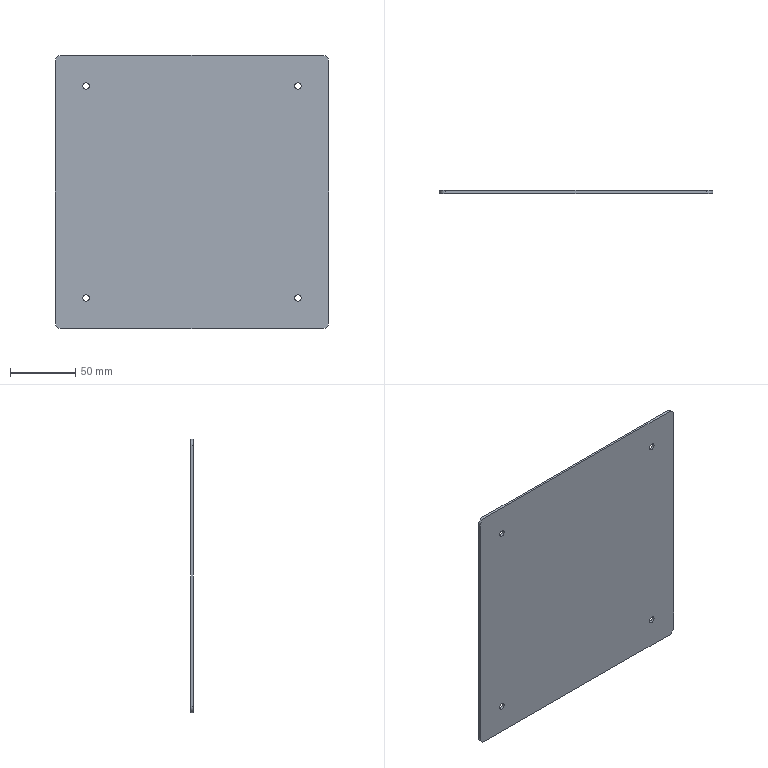Part | SolidWorks | features Extrusion 1, Fillet 1, HoleWzd 1 | 1 solid | 18 faces | box 210 x 2 x 210 mm | volume 88000 mm3 | cylinder 12 | plane 6 | commonest cylinder face diameters 5 x8 10 x4
STEP:
#1=CARTESIAN_POINT('',(-81.317,0.,78.817));
#2=VERTEX_POINT('',#1);
#3=CARTESIAN_POINT('',(-81.317,0.,83.817));
#4=VERTEX_POINT('',#3);
#5=CARTESIAN_POINT('',(-81.317,0.,81.317));
#6=DIRECTION('',(0.,1.,0.));
#7=DIRECTION('',(0.,0.,1.));
#8=AXIS2_PLACEMENT_3D('',#5,#6,#7);
#9=CIRCLE('',#8,2.5);
#10=EDGE_CURVE('',#2,#4,#9,.T.);
#11=ORIENTED_EDGE('',*,*,#10,.F.);
#12=CARTESIAN_POINT('',(-81.317,2.,78.817));
#13=VERTEX_POINT('',#12);
#14=CARTESIAN_POINT('',(-81.317,2.,78.817));
#15=DIRECTION('',(0.,1.,0.));
#16=VECTOR('',#15,1000.);
#17=LINE('',#14,#16);
#18=EDGE_CURVE('',#2,#13,#17,.T.);
#19=ORIENTED_EDGE('',*,*,#18,.T.);
#20=CARTESIAN_POINT('',(-81.317,2.,83.817));
#21=VERTEX_POINT('',#20);
#22=CARTESIAN_POINT('',(-81.317,2.,81.317));
#23=DIRECTION('',(0.,1.,0.));
#24=DIRECTION('',(0.,0.,1.));
#25=AXIS2_PLACEMENT_3D('',#22,#23,#24);
#26=CIRCLE('',#25,2.5);
#27=EDGE_CURVE('',#13,#21,#26,.T.);
#28=ORIENTED_EDGE('',*,*,#27,.T.);
#29=CARTESIAN_POINT('',(-81.317,2.,83.817));
#30=DIRECTION('',(0.,1.,0.));
#31=VECTOR('',#30,1000.);
#32=LINE('',#29,#31);
#33=EDGE_CURVE('',#4,#21,#32,.T.);
#34=ORIENTED_EDGE('',*,*,#33,.F.);
#35=EDGE_LOOP('',(#11,#19,#28,#34));
#36=FACE_OUTER_BOUND('',#35,.T.);
#37=CARTESIAN_POINT('',(-81.317,2.,81.317));
#38=DIRECTION('',(0.,1.,0.));
#39=DIRECTION('',(0.,0.,1.));
#40=AXIS2_PLACEMENT_3D('',#37,#38,#39);
#41=CYLINDRICAL_SURFACE('',#40,2.5);
#42=ADVANCED_FACE('',(#36),#41,.F.);
#43=CARTESIAN_POINT('',(-81.317,0.,-83.817));
#44=VERTEX_POINT('',#43);
#45=CARTESIAN_POINT('',(-81.317,0.,-78.817));
#46=VERTEX_POINT('',#45);
#47=CARTESIAN_POINT('',(-81.317,0.,-81.317));
#48=DIRECTION('',(0.,1.,0.));
#49=DIRECTION('',(0.,0.,1.));
#50=AXIS2_PLACEMENT_3D('',#47,#48,#49);
#51=CIRCLE('',#50,2.5);
#52=EDGE_CURVE('',#44,#46,#51,.T.);
#53=ORIENTED_EDGE('',*,*,#52,.F.);
#54=CARTESIAN_POINT('',(-81.317,2.,-83.817));
#55=VERTEX_POINT('',#54);
#56=CARTESIAN_POINT('',(-81.317,2.,-83.817));
#57=DIRECTION('',(0.,1.,0.));
#58=VECTOR('',#57,1000.);
#59=LINE('',#56,#58);
#60=EDGE_CURVE('',#44,#55,#59,.T.);
#61=ORIENTED_EDGE('',*,*,#60,.T.);
#62=CARTESIAN_POINT('',(-81.317,2.,-78.817));
#63=VERTEX_POINT('',#62);
#64=CARTESIAN_POINT('',(-81.317,2.,-81.317));
#65=DIRECTION('',(0.,1.,0.));
#66=DIRECTION('',(0.,0.,1.));
#67=AXIS2_PLACEMENT_3D('',#64,#65,#66);
#68=CIRCLE('',#67,2.5);
#69=EDGE_CURVE('',#55,#63,#68,.T.);
#70=ORIENTED_EDGE('',*,*,#69,.T.);
#71=CARTESIAN_POINT('',(-81.317,2.,-78.817));
#72=DIRECTION('',(0.,1.,0.));
#73=VECTOR('',#72,1000.);
#74=LINE('',#71,#73);
#75=EDGE_CURVE('',#46,#63,#74,.T.);
#76=ORIENTED_EDGE('',*,*,#75,.F.);
#77=EDGE_LOOP('',(#53,#61,#70,#76));
#78=FACE_OUTER_BOUND('',#77,.T.);
#79=CARTESIAN_POINT('',(-81.317,2.,-81.317));
#80=DIRECTION('',(0.,1.,0.));
#81=DIRECTION('',(0.,0.,1.));
#82=AXIS2_PLACEMENT_3D('',#79,#80,#81);
#83=CYLINDRICAL_SURFACE('',#82,2.5);
#84=ADVANCED_FACE('',(#78),#83,.F.);
#85=CARTESIAN_POINT('',(81.317,0.,-83.817));
#86=VERTEX_POINT('',#85);
#87=CARTESIAN_POINT('',(81.317,0.,-78.817));
#88=VERTEX_POINT('',#87);
#89=CARTESIAN_POINT('',(81.317,0.,-81.317));
#90=DIRECTION('',(0.,1.,0.));
#91=DIRECTION('',(0.,0.,1.));
#92=AXIS2_PLACEMENT_3D('',#89,#90,#91);
#93=CIRCLE('',#92,2.5);
#94=EDGE_CURVE('',#86,#88,#93,.T.);
#95=ORIENTED_EDGE('',*,*,#94,.F.);
#96=CARTESIAN_POINT('',(81.317,2.,-83.817));
#97=VERTEX_POINT('',#96);
#98=CARTESIAN_POINT('',(81.317,2.,-83.817));
#99=DIRECTION('',(0.,1.,0.));
#100=VECTOR('',#99,1000.);
#101=LINE('',#98,#100);
#102=EDGE_CURVE('',#86,#97,#101,.T.);
#103=ORIENTED_EDGE('',*,*,#102,.T.);
#104=CARTESIAN_POINT('',(81.317,2.,-78.817));
#105=VERTEX_POINT('',#104);
#106=CARTESIAN_POINT('',(81.317,2.,-81.317));
#107=DIRECTION('',(0.,1.,0.));
#108=DIRECTION('',(0.,0.,1.));
#109=AXIS2_PLACEMENT_3D('',#106,#107,#108);
#110=CIRCLE('',#109,2.5);
#111=EDGE_CURVE('',#97,#105,#110,.T.);
#112=ORIENTED_EDGE('',*,*,#111,.T.);
#113=CARTESIAN_POINT('',(81.317,2.,-78.817));
#114=DIRECTION('',(0.,1.,0.));
#115=VECTOR('',#114,1000.);
#116=LINE('',#113,#115);
#117=EDGE_CURVE('',#88,#105,#116,.T.);
#118=ORIENTED_EDGE('',*,*,#117,.F.);
#119=EDGE_LOOP('',(#95,#103,#112,#118));
#120=FACE_OUTER_BOUND('',#119,.T.);
#121=CARTESIAN_POINT('',(81.317,2.,-81.317));
#122=DIRECTION('',(0.,1.,0.));
#123=DIRECTION('',(0.,0.,1.));
#124=AXIS2_PLACEMENT_3D('',#121,#122,#123);
#125=CYLINDRICAL_SURFACE('',#124,2.5);
#126=ADVANCED_FACE('',(#120),#125,.F.);
#127=CARTESIAN_POINT('',(81.317,0.,78.817));
#128=VERTEX_POINT('',#127);
#129=CARTESIAN_POINT('',(81.317,0.,83.817));
#130=VERTEX_POINT('',#129);
#131=CARTESIAN_POINT('',(81.317,0.,81.317));
#132=DIRECTION('',(0.,1.,0.));
#133=DIRECTION('',(0.,0.,1.));
#134=AXIS2_PLACEMENT_3D('',#131,#132,#133);
#135=CIRCLE('',#134,2.5);
#136=EDGE_CURVE('',#128,#130,#135,.T.);
#137=ORIENTED_EDGE('',*,*,#136,.F.);
#138=CARTESIAN_POINT('',(81.317,2.,78.817));
#139=VERTEX_POINT('',#138);
#140=CARTESIAN_POINT('',(81.317,2.,78.817));
#141=DIRECTION('',(0.,1.,0.));
#142=VECTOR('',#141,1000.);
#143=LINE('',#140,#142);
#144=EDGE_CURVE('',#128,#139,#143,.T.);
#145=ORIENTED_EDGE('',*,*,#144,.T.);
#146=CARTESIAN_POINT('',(81.317,2.,83.817));
#147=VERTEX_POINT('',#146);
#148=CARTESIAN_POINT('',(81.317,2.,81.317));
#149=DIRECTION('',(0.,1.,0.));
#150=DIRECTION('',(0.,0.,1.));
#151=AXIS2_PLACEMENT_3D('',#148,#149,#150);
#152=CIRCLE('',#151,2.5);
#153=EDGE_CURVE('',#139,#147,#152,.T.);
#154=ORIENTED_EDGE('',*,*,#153,.T.);
#155=CARTESIAN_POINT('',(81.317,2.,83.817));
#156=DIRECTION('',(0.,1.,0.));
#157=VECTOR('',#156,1000.);
#158=LINE('',#155,#157);
#159=EDGE_CURVE('',#130,#147,#158,.T.);
#160=ORIENTED_EDGE('',*,*,#159,.F.);
#161=EDGE_LOOP('',(#137,#145,#154,#160));
#162=FACE_OUTER_BOUND('',#161,.T.);
#163=CARTESIAN_POINT('',(81.317,2.,81.317));
#164=DIRECTION('',(0.,1.,0.));
#165=DIRECTION('',(0.,0.,1.));
#166=AXIS2_PLACEMENT_3D('',#163,#164,#165);
#167=CYLINDRICAL_SURFACE('',#166,2.5);
#168=ADVANCED_FACE('',(#162),#167,.F.);
#169=CARTESIAN_POINT('',(105.,2.,100.));
#170=VERTEX_POINT('',#169);
#171=CARTESIAN_POINT('',(105.,2.,-100.));
#172=VERTEX_POINT('',#171);
#173=CARTESIAN_POINT('',(105.,2.,-105.));
#174=DIRECTION('',(0.,0.,-1.));
#175=VECTOR('',#174,1000.);
#176=LINE('',#173,#175);
#177=EDGE_CURVE('',#170,#172,#176,.T.);
#178=ORIENTED_EDGE('',*,*,#177,.F.);
#179=CARTESIAN_POINT('',(105.,0.,100.));
#180=VERTEX_POINT('',#179);
#181=CARTESIAN_POINT('',(105.,2.,100.));
#182=DIRECTION('',(0.,-1.,0.));
#183=VECTOR('',#182,1000.);
#184=LINE('',#181,#183);
#185=EDGE_CURVE('',#170,#180,#184,.T.);
#186=ORIENTED_EDGE('',*,*,#185,.T.);
#187=CARTESIAN_POINT('',(105.,0.,-100.));
#188=VERTEX_POINT('',#187);
#189=CARTESIAN_POINT('',(105.,0.,-105.));
#190=DIRECTION('',(0.,0.,-1.));
#191=VECTOR('',#190,1000.);
#192=LINE('',#189,#191);
#193=EDGE_CURVE('',#180,#188,#192,.T.);
#194=ORIENTED_EDGE('',*,*,#193,.T.);
#195=CARTESIAN_POINT('',(105.,2.,-100.));
#196=DIRECTION('',(0.,1.,0.));
#197=VECTOR('',#196,1000.);
#198=LINE('',#195,#197);
#199=EDGE_CURVE('',#188,#172,#198,.T.);
#200=ORIENTED_EDGE('',*,*,#199,.T.);
#201=EDGE_LOOP('',(#178,#186,#194,#200));
#202=FACE_OUTER_BOUND('',#201,.T.);
#203=CARTESIAN_POINT('',(105.,2.,-105.));
#204=DIRECTION('',(-1.,0.,0.));
#205=DIRECTION('',(0.,0.,1.));
#206=AXIS2_PLACEMENT_3D('',#203,#204,#205);
#207=PLANE('',#206);
#208=ADVANCED_FACE('',(#202),#207,.F.);
#209=CARTESIAN_POINT('',(100.,0.,-105.));
#210=VERTEX_POINT('',#209);
#211=CARTESIAN_POINT('',(-100.,0.,-105.));
#212=VERTEX_POINT('',#211);
#213=CARTESIAN_POINT('',(-105.,0.,-105.));
#214=DIRECTION('',(-1.,0.,0.));
#215=VECTOR('',#214,1000.);
#216=LINE('',#213,#215);
#217=EDGE_CURVE('',#210,#212,#216,.T.);
#218=ORIENTED_EDGE('',*,*,#217,.T.);
#219=CARTESIAN_POINT('',(-100.,2.,-105.));
#220=VERTEX_POINT('',#219);
#221=CARTESIAN_POINT('',(-100.,2.,-105.));
#222=DIRECTION('',(0.,1.,0.));
#223=VECTOR('',#222,1000.);
#224=LINE('',#221,#223);
#225=EDGE_CURVE('',#212,#220,#224,.T.);
#226=ORIENTED_EDGE('',*,*,#225,.T.);
#227=CARTESIAN_POINT('',(100.,2.,-105.));
#228=VERTEX_POINT('',#227);
#229=CARTESIAN_POINT('',(-105.,2.,-105.));
#230=DIRECTION('',(-1.,0.,0.));
#231=VECTOR('',#230,1000.);
#232=LINE('',#229,#231);
#233=EDGE_CURVE('',#228,#220,#232,.T.);
#234=ORIENTED_EDGE('',*,*,#233,.F.);
#235=CARTESIAN_POINT('',(100.,2.,-105.));
#236=DIRECTION('',(0.,-1.,0.));
#237=VECTOR('',#236,1000.);
#238=LINE('',#235,#237);
#239=EDGE_CURVE('',#228,#210,#238,.T.);
#240=ORIENTED_EDGE('',*,*,#239,.T.);
#241=EDGE_LOOP('',(#218,#226,#234,#240));
#242=FACE_OUTER_BOUND('',#241,.T.);
#243=CARTESIAN_POINT('',(-105.,2.,-105.));
#244=DIRECTION('',(0.,0.,1.));
#245=DIRECTION('',(1.,0.,0.));
#246=AXIS2_PLACEMENT_3D('',#243,#244,#245);
#247=PLANE('',#246);
#248=ADVANCED_FACE('',(#242),#247,.F.);
#249=CARTESIAN_POINT('',(-105.,2.,-100.));
#250=VERTEX_POINT('',#249);
#251=CARTESIAN_POINT('',(-105.,2.,100.));
#252=VERTEX_POINT('',#251);
#253=CARTESIAN_POINT('',(-105.,2.,-105.));
#254=DIRECTION('',(0.,0.,1.));
#255=VECTOR('',#254,1000.);
#256=LINE('',#253,#255);
#257=EDGE_CURVE('',#250,#252,#256,.T.);
#258=ORIENTED_EDGE('',*,*,#257,.F.);
#259=CARTESIAN_POINT('',(-105.,0.,-100.));
#260=VERTEX_POINT('',#259);
#261=CARTESIAN_POINT('',(-105.,2.,-100.));
#262=DIRECTION('',(0.,-1.,0.));
#263=VECTOR('',#262,1000.);
#264=LINE('',#261,#263);
#265=EDGE_CURVE('',#250,#260,#264,.T.);
#266=ORIENTED_EDGE('',*,*,#265,.T.);
#267=CARTESIAN_POINT('',(-105.,0.,100.));
#268=VERTEX_POINT('',#267);
#269=CARTESIAN_POINT('',(-105.,0.,-105.));
#270=DIRECTION('',(0.,0.,1.));
#271=VECTOR('',#270,1000.);
#272=LINE('',#269,#271);
#273=EDGE_CURVE('',#260,#268,#272,.T.);
#274=ORIENTED_EDGE('',*,*,#273,.T.);
#275=CARTESIAN_POINT('',(-105.,2.,100.));
#276=DIRECTION('',(0.,1.,0.));
#277=VECTOR('',#276,1000.);
#278=LINE('',#275,#277);
#279=EDGE_CURVE('',#268,#252,#278,.T.);
#280=ORIENTED_EDGE('',*,*,#279,.T.);
#281=EDGE_LOOP('',(#258,#266,#274,#280));
#282=FACE_OUTER_BOUND('',#281,.T.);
#283=CARTESIAN_POINT('',(-105.,2.,-105.));
#284=DIRECTION('',(1.,0.,0.));
#285=DIRECTION('',(0.,0.,-1.));
#286=AXIS2_PLACEMENT_3D('',#283,#284,#285);
#287=PLANE('',#286);
#288=ADVANCED_FACE('',(#282),#287,.F.);
#289=CARTESIAN_POINT('',(-100.,0.,105.));
#290=VERTEX_POINT('',#289);
#291=CARTESIAN_POINT('',(100.,0.,105.));
#292=VERTEX_POINT('',#291);
#293=CARTESIAN_POINT('',(-105.,0.,105.));
#294=DIRECTION('',(1.,0.,0.));
#295=VECTOR('',#294,1000.);
#296=LINE('',#293,#295);
#297=EDGE_CURVE('',#290,#292,#296,.T.);
#298=ORIENTED_EDGE('',*,*,#297,.T.);
#299=CARTESIAN_POINT('',(100.,2.,105.));
#300=VERTEX_POINT('',#299);
#301=CARTESIAN_POINT('',(100.,2.,105.));
#302=DIRECTION('',(0.,1.,0.));
#303=VECTOR('',#302,1000.);
#304=LINE('',#301,#303);
#305=EDGE_CURVE('',#292,#300,#304,.T.);
#306=ORIENTED_EDGE('',*,*,#305,.T.);
#307=CARTESIAN_POINT('',(-100.,2.,105.));
#308=VERTEX_POINT('',#307);
#309=CARTESIAN_POINT('',(-105.,2.,105.));
#310=DIRECTION('',(1.,0.,0.));
#311=VECTOR('',#310,1000.);
#312=LINE('',#309,#311);
#313=EDGE_CURVE('',#308,#300,#312,.T.);
#314=ORIENTED_EDGE('',*,*,#313,.F.);
#315=CARTESIAN_POINT('',(-100.,2.,105.));
#316=DIRECTION('',(0.,-1.,0.));
#317=VECTOR('',#316,1000.);
#318=LINE('',#315,#317);
#319=EDGE_CURVE('',#308,#290,#318,.T.);
#320=ORIENTED_EDGE('',*,*,#319,.T.);
#321=EDGE_LOOP('',(#298,#306,#314,#320));
#322=FACE_OUTER_BOUND('',#321,.T.);
#323=CARTESIAN_POINT('',(-105.,2.,105.));
#324=DIRECTION('',(0.,0.,-1.));
#325=DIRECTION('',(-1.,0.,0.));
#326=AXIS2_PLACEMENT_3D('',#323,#324,#325);
#327=PLANE('',#326);
#328=ADVANCED_FACE('',(#322),#327,.F.);
#329=CARTESIAN_POINT('',(-81.317,2.,81.317));
#330=DIRECTION('',(0.,1.,0.));
#331=DIRECTION('',(0.,0.,1.));
#332=AXIS2_PLACEMENT_3D('',#329,#330,#331);
#333=CIRCLE('',#332,2.5);
#334=EDGE_CURVE('',#21,#13,#333,.T.);
#335=ORIENTED_EDGE('',*,*,#334,.F.);
#336=ORIENTED_EDGE('',*,*,#27,.F.);
#337=EDGE_LOOP('',(#335,#336));
#338=FACE_BOUND('',#337,.T.);
#339=CARTESIAN_POINT('',(-81.317,2.,-81.317));
#340=DIRECTION('',(0.,1.,0.));
#341=DIRECTION('',(0.,0.,1.));
#342=AXIS2_PLACEMENT_3D('',#339,#340,#341);
#343=CIRCLE('',#342,2.5);
#344=EDGE_CURVE('',#63,#55,#343,.T.);
#345=ORIENTED_EDGE('',*,*,#344,.F.);
#346=ORIENTED_EDGE('',*,*,#69,.F.);
#347=EDGE_LOOP('',(#345,#346));
#348=FACE_BOUND('',#347,.T.);
#349=CARTESIAN_POINT('',(81.317,2.,-81.317));
#350=DIRECTION('',(0.,1.,0.));
#351=DIRECTION('',(0.,0.,1.));
#352=AXIS2_PLACEMENT_3D('',#349,#350,#351);
#353=CIRCLE('',#352,2.5);
#354=EDGE_CURVE('',#105,#97,#353,.T.);
#355=ORIENTED_EDGE('',*,*,#354,.F.);
#356=ORIENTED_EDGE('',*,*,#111,.F.);
#357=EDGE_LOOP('',(#355,#356));
#358=FACE_BOUND('',#357,.T.);
#359=CARTESIAN_POINT('',(81.317,2.,81.317));
#360=DIRECTION('',(0.,1.,0.));
#361=DIRECTION('',(0.,0.,1.));
#362=AXIS2_PLACEMENT_3D('',#359,#360,#361);
#363=CIRCLE('',#362,2.5);
#364=EDGE_CURVE('',#147,#139,#363,.T.);
#365=ORIENTED_EDGE('',*,*,#364,.F.);
#366=ORIENTED_EDGE('',*,*,#153,.F.);
#367=EDGE_LOOP('',(#365,#366));
#368=FACE_BOUND('',#367,.T.);
#369=ORIENTED_EDGE('',*,*,#313,.T.);
#370=CARTESIAN_POINT('',(100.,2.,100.));
#371=DIRECTION('',(0.,1.,0.));
#372=DIRECTION('',(0.,0.,1.));
#373=AXIS2_PLACEMENT_3D('',#370,#371,#372);
#374=CIRCLE('',#373,5.);
#375=EDGE_CURVE('',#300,#170,#374,.T.);
#376=ORIENTED_EDGE('',*,*,#375,.T.);
#377=ORIENTED_EDGE('',*,*,#177,.T.);
#378=CARTESIAN_POINT('',(100.,2.,-100.));
#379=DIRECTION('',(0.,1.,0.));
#380=DIRECTION('',(0.,0.,1.));
#381=AXIS2_PLACEMENT_3D('',#378,#379,#380);
#382=CIRCLE('',#381,5.);
#383=EDGE_CURVE('',#172,#228,#382,.T.);
#384=ORIENTED_EDGE('',*,*,#383,.T.);
#385=ORIENTED_EDGE('',*,*,#233,.T.);
#386=CARTESIAN_POINT('',(-100.,2.,-100.));
#387=DIRECTION('',(0.,1.,0.));
#388=DIRECTION('',(0.,0.,1.));
#389=AXIS2_PLACEMENT_3D('',#386,#387,#388);
#390=CIRCLE('',#389,5.);
#391=EDGE_CURVE('',#220,#250,#390,.T.);
#392=ORIENTED_EDGE('',*,*,#391,.T.);
#393=ORIENTED_EDGE('',*,*,#257,.T.);
#394=CARTESIAN_POINT('',(-100.,2.,100.));
#395=DIRECTION('',(0.,1.,0.));
#396=DIRECTION('',(0.,0.,1.));
#397=AXIS2_PLACEMENT_3D('',#394,#395,#396);
#398=CIRCLE('',#397,5.);
#399=EDGE_CURVE('',#252,#308,#398,.T.);
#400=ORIENTED_EDGE('',*,*,#399,.T.);
#401=EDGE_LOOP('',(#369,#376,#377,#384,#385,#392,#393,#400));
#402=FACE_OUTER_BOUND('',#401,.T.);
#403=CARTESIAN_POINT('',(0.,2.,0.));
#404=DIRECTION('',(0.,1.,0.));
#405=DIRECTION('',(0.,0.,1.));
#406=AXIS2_PLACEMENT_3D('',#403,#404,#405);
#407=PLANE('',#406);
#408=ADVANCED_FACE('',(#338,#348,#358,#368,#402),#407,.T.);
#409=CARTESIAN_POINT('',(-81.317,0.,81.317));
#410=DIRECTION('',(0.,1.,0.));
#411=DIRECTION('',(0.,0.,1.));
#412=AXIS2_PLACEMENT_3D('',#409,#410,#411);
#413=CIRCLE('',#412,2.5);
#414=EDGE_CURVE('',#4,#2,#413,.T.);
#415=ORIENTED_EDGE('',*,*,#414,.T.);
#416=ORIENTED_EDGE('',*,*,#10,.T.);
#417=EDGE_LOOP('',(#415,#416));
#418=FACE_BOUND('',#417,.T.);
#419=CARTESIAN_POINT('',(-81.317,0.,-81.317));
#420=DIRECTION('',(0.,1.,0.));
#421=DIRECTION('',(0.,0.,1.));
#422=AXIS2_PLACEMENT_3D('',#419,#420,#421);
#423=CIRCLE('',#422,2.5);
#424=EDGE_CURVE('',#46,#44,#423,.T.);
#425=ORIENTED_EDGE('',*,*,#424,.T.);
#426=ORIENTED_EDGE('',*,*,#52,.T.);
#427=EDGE_LOOP('',(#425,#426));
#428=FACE_BOUND('',#427,.T.);
#429=CARTESIAN_POINT('',(81.317,0.,-81.317));
#430=DIRECTION('',(0.,1.,0.));
#431=DIRECTION('',(0.,0.,1.));
#432=AXIS2_PLACEMENT_3D('',#429,#430,#431);
#433=CIRCLE('',#432,2.5);
#434=EDGE_CURVE('',#88,#86,#433,.T.);
#435=ORIENTED_EDGE('',*,*,#434,.T.);
#436=ORIENTED_EDGE('',*,*,#94,.T.);
#437=EDGE_LOOP('',(#435,#436));
#438=FACE_BOUND('',#437,.T.);
#439=CARTESIAN_POINT('',(81.317,0.,81.317));
#440=DIRECTION('',(0.,1.,0.));
#441=DIRECTION('',(0.,0.,1.));
#442=AXIS2_PLACEMENT_3D('',#439,#440,#441);
#443=CIRCLE('',#442,2.5);
#444=EDGE_CURVE('',#130,#128,#443,.T.);
#445=ORIENTED_EDGE('',*,*,#444,.T.);
#446=ORIENTED_EDGE('',*,*,#136,.T.);
#447=EDGE_LOOP('',(#445,#446));
#448=FACE_BOUND('',#447,.T.);
#449=ORIENTED_EDGE('',*,*,#193,.F.);
#450=CARTESIAN_POINT('',(100.,0.,100.));
#451=DIRECTION('',(0.,-1.,0.));
#452=DIRECTION('',(0.,0.,1.));
#453=AXIS2_PLACEMENT_3D('',#450,#451,#452);
#454=CIRCLE('',#453,5.);
#455=EDGE_CURVE('',#180,#292,#454,.T.);
#456=ORIENTED_EDGE('',*,*,#455,.T.);
#457=ORIENTED_EDGE('',*,*,#297,.F.);
#458=CARTESIAN_POINT('',(-100.,0.,100.));
#459=DIRECTION('',(0.,-1.,0.));
#460=DIRECTION('',(0.,0.,1.));
#461=AXIS2_PLACEMENT_3D('',#458,#459,#460);
#462=CIRCLE('',#461,5.);
#463=EDGE_CURVE('',#290,#268,#462,.T.);
#464=ORIENTED_EDGE('',*,*,#463,.T.);
#465=ORIENTED_EDGE('',*,*,#273,.F.);
#466=CARTESIAN_POINT('',(-100.,0.,-100.));
#467=DIRECTION('',(0.,-1.,0.));
#468=DIRECTION('',(0.,0.,1.));
#469=AXIS2_PLACEMENT_3D('',#466,#467,#468);
#470=CIRCLE('',#469,5.);
#471=EDGE_CURVE('',#260,#212,#470,.T.);
#472=ORIENTED_EDGE('',*,*,#471,.T.);
#473=ORIENTED_EDGE('',*,*,#217,.F.);
#474=CARTESIAN_POINT('',(100.,0.,-100.));
#475=DIRECTION('',(0.,-1.,0.));
#476=DIRECTION('',(0.,0.,1.));
#477=AXIS2_PLACEMENT_3D('',#474,#475,#476);
#478=CIRCLE('',#477,5.);
#479=EDGE_CURVE('',#210,#188,#478,.T.);
#480=ORIENTED_EDGE('',*,*,#479,.T.);
#481=EDGE_LOOP('',(#449,#456,#457,#464,#465,#472,#473,#480));
#482=FACE_OUTER_BOUND('',#481,.T.);
#483=CARTESIAN_POINT('',(0.,0.,0.));
#484=DIRECTION('',(0.,1.,0.));
#485=DIRECTION('',(0.,0.,1.));
#486=AXIS2_PLACEMENT_3D('',#483,#484,#485);
#487=PLANE('',#486);
#488=ADVANCED_FACE('',(#418,#428,#438,#448,#482),#487,.F.);
#489=ORIENTED_EDGE('',*,*,#144,.F.);
#490=ORIENTED_EDGE('',*,*,#444,.F.);
#491=ORIENTED_EDGE('',*,*,#159,.T.);
#492=ORIENTED_EDGE('',*,*,#364,.T.);
#493=EDGE_LOOP('',(#489,#490,#491,#492));
#494=FACE_OUTER_BOUND('',#493,.T.);
#495=CARTESIAN_POINT('',(81.317,2.,81.317));
#496=DIRECTION('',(0.,1.,0.));
#497=DIRECTION('',(0.,0.,1.));
#498=AXIS2_PLACEMENT_3D('',#495,#496,#497);
#499=CYLINDRICAL_SURFACE('',#498,2.5);
#500=ADVANCED_FACE('',(#494),#499,.F.);
#501=ORIENTED_EDGE('',*,*,#102,.F.);
#502=ORIENTED_EDGE('',*,*,#434,.F.);
#503=ORIENTED_EDGE('',*,*,#117,.T.);
#504=ORIENTED_EDGE('',*,*,#354,.T.);
#505=EDGE_LOOP('',(#501,#502,#503,#504));
#506=FACE_OUTER_BOUND('',#505,.T.);
#507=CARTESIAN_POINT('',(81.317,2.,-81.317));
#508=DIRECTION('',(0.,1.,0.));
#509=DIRECTION('',(0.,0.,1.));
#510=AXIS2_PLACEMENT_3D('',#507,#508,#509);
#511=CYLINDRICAL_SURFACE('',#510,2.5);
#512=ADVANCED_FACE('',(#506),#511,.F.);
#513=ORIENTED_EDGE('',*,*,#60,.F.);
#514=ORIENTED_EDGE('',*,*,#424,.F.);
#515=ORIENTED_EDGE('',*,*,#75,.T.);
#516=ORIENTED_EDGE('',*,*,#344,.T.);
#517=EDGE_LOOP('',(#513,#514,#515,#516));
#518=FACE_OUTER_BOUND('',#517,.T.);
#519=CARTESIAN_POINT('',(-81.317,2.,-81.317));
#520=DIRECTION('',(0.,1.,0.));
#521=DIRECTION('',(0.,0.,1.));
#522=AXIS2_PLACEMENT_3D('',#519,#520,#521);
#523=CYLINDRICAL_SURFACE('',#522,2.5);
#524=ADVANCED_FACE('',(#518),#523,.F.);
#525=ORIENTED_EDGE('',*,*,#18,.F.);
#526=ORIENTED_EDGE('',*,*,#414,.F.);
#527=ORIENTED_EDGE('',*,*,#33,.T.);
#528=ORIENTED_EDGE('',*,*,#334,.T.);
#529=EDGE_LOOP('',(#525,#526,#527,#528));
#530=FACE_OUTER_BOUND('',#529,.T.);
#531=CARTESIAN_POINT('',(-81.317,2.,81.317));
#532=DIRECTION('',(0.,1.,0.));
#533=DIRECTION('',(0.,0.,1.));
#534=AXIS2_PLACEMENT_3D('',#531,#532,#533);
#535=CYLINDRICAL_SURFACE('',#534,2.5);
#536=ADVANCED_FACE('',(#530),#535,.F.);
#537=ORIENTED_EDGE('',*,*,#375,.F.);
#538=ORIENTED_EDGE('',*,*,#305,.F.);
#539=ORIENTED_EDGE('',*,*,#455,.F.);
#540=ORIENTED_EDGE('',*,*,#185,.F.);
#541=EDGE_LOOP('',(#537,#538,#539,#540));
#542=FACE_OUTER_BOUND('',#541,.T.);
#543=CARTESIAN_POINT('',(100.,2.,100.));
#544=DIRECTION('',(0.,-1.,0.));
#545=DIRECTION('',(0.,0.,-1.));
#546=AXIS2_PLACEMENT_3D('',#543,#544,#545);
#547=CYLINDRICAL_SURFACE('',#546,5.);
#548=ADVANCED_FACE('',(#542),#547,.T.);
#549=ORIENTED_EDGE('',*,*,#391,.F.);
#550=ORIENTED_EDGE('',*,*,#225,.F.);
#551=ORIENTED_EDGE('',*,*,#471,.F.);
#552=ORIENTED_EDGE('',*,*,#265,.F.);
#553=EDGE_LOOP('',(#549,#550,#551,#552));
#554=FACE_OUTER_BOUND('',#553,.T.);
#555=CARTESIAN_POINT('',(-100.,2.,-100.));
#556=DIRECTION('',(0.,-1.,0.));
#557=DIRECTION('',(0.,0.,-1.));
#558=AXIS2_PLACEMENT_3D('',#555,#556,#557);
#559=CYLINDRICAL_SURFACE('',#558,5.);
#560=ADVANCED_FACE('',(#554),#559,.T.);
#561=ORIENTED_EDGE('',*,*,#383,.F.);
#562=ORIENTED_EDGE('',*,*,#199,.F.);
#563=ORIENTED_EDGE('',*,*,#479,.F.);
#564=ORIENTED_EDGE('',*,*,#239,.F.);
#565=EDGE_LOOP('',(#561,#562,#563,#564));
#566=FACE_OUTER_BOUND('',#565,.T.);
#567=CARTESIAN_POINT('',(100.,2.,-100.));
#568=DIRECTION('',(0.,-1.,0.));
#569=DIRECTION('',(0.,0.,-1.));
#570=AXIS2_PLACEMENT_3D('',#567,#568,#569);
#571=CYLINDRICAL_SURFACE('',#570,5.);
#572=ADVANCED_FACE('',(#566),#571,.T.);
#573=ORIENTED_EDGE('',*,*,#399,.F.);
#574=ORIENTED_EDGE('',*,*,#279,.F.);
#575=ORIENTED_EDGE('',*,*,#463,.F.);
#576=ORIENTED_EDGE('',*,*,#319,.F.);
#577=EDGE_LOOP('',(#573,#574,#575,#576));
#578=FACE_OUTER_BOUND('',#577,.T.);
#579=CARTESIAN_POINT('',(-100.,2.,100.));
#580=DIRECTION('',(0.,-1.,0.));
#581=DIRECTION('',(0.,0.,-1.));
#582=AXIS2_PLACEMENT_3D('',#579,#580,#581);
#583=CYLINDRICAL_SURFACE('',#582,5.);
#584=ADVANCED_FACE('',(#578),#583,.T.);
#585=CLOSED_SHELL('',(#42,#84,#126,#168,#208,#248,#288,#328,#408,#488,#500,#512,#524,#536,#548,#560,#572,#584));
#586=MANIFOLD_SOLID_BREP('',#585);
#587=CARTESIAN_POINT('',(0.,0.,0.));
#588=DIRECTION('',(0.,0.,1.));
#589=DIRECTION('',(1.,0.,0.));
#590=AXIS2_PLACEMENT_3D('',#587,#588,#589);
#591=(LENGTH_UNIT()NAMED_UNIT(*)SI_UNIT(.MILLI.,.METRE.));
#592=UNCERTAINTY_MEASURE_WITH_UNIT(LENGTH_MEASURE(0.00001),#591,'','');
#593=(NAMED_UNIT(*)PLANE_ANGLE_UNIT()SI_UNIT($,.RADIAN.));
#594=(NAMED_UNIT(*)SI_UNIT($,.STERADIAN.)SOLID_ANGLE_UNIT());
#595=(GEOMETRIC_REPRESENTATION_CONTEXT(3)GLOBAL_UNCERTAINTY_ASSIGNED_CONTEXT((#592))GLOBAL_UNIT_ASSIGNED_CONTEXT((#591,#593,#594))REPRESENTATION_CONTEXT('',''));
#596=ADVANCED_BREP_SHAPE_REPRESENTATION('',(#586,#590),#595);